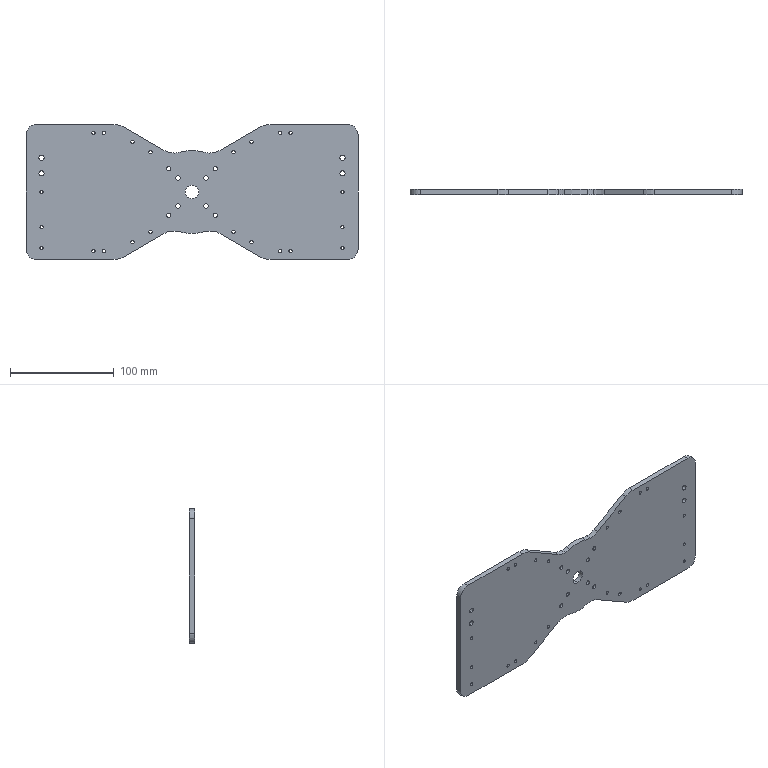Part | SolidWorks | features BaseBody 1 | 1 solid | 99 faces | box 320 x 5 x 130 mm | volume 180155 mm3 | cylinder 87 | plane 12 | commonest cylinder face diameters 3.2 x44 4.2 x16 40 x10 5 x8 20 x4 80 x3